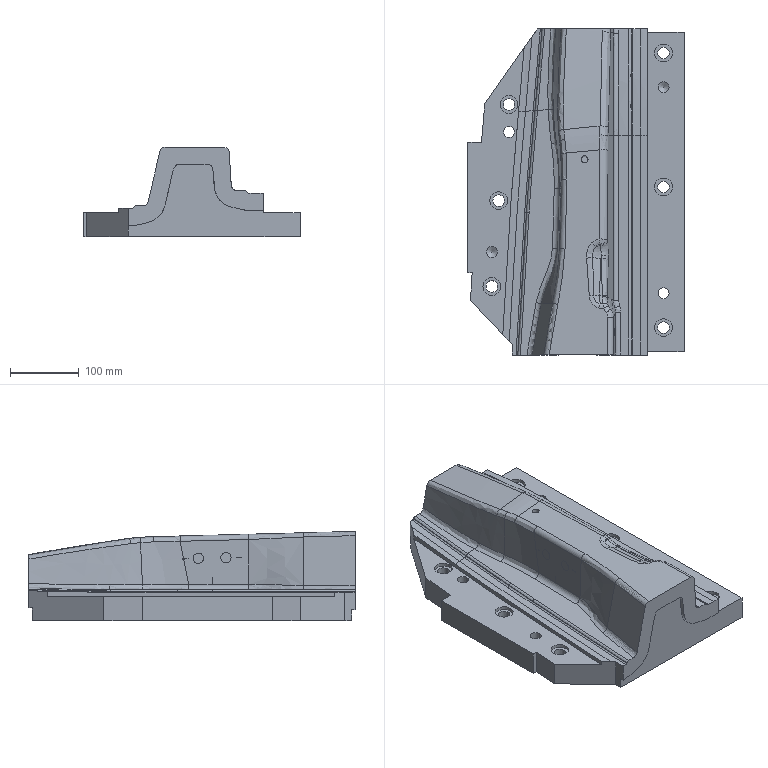Part | NX | features solid 2 | 1 solid | 163 faces | box 315 x 475 x 129.892 mm | volume 8006583 mm3 | spline 116 | plane 28 | cylinder 17 | cone 2 | commonest cylinder face diameters 17 x6 26 x6 16 x4 10 x1